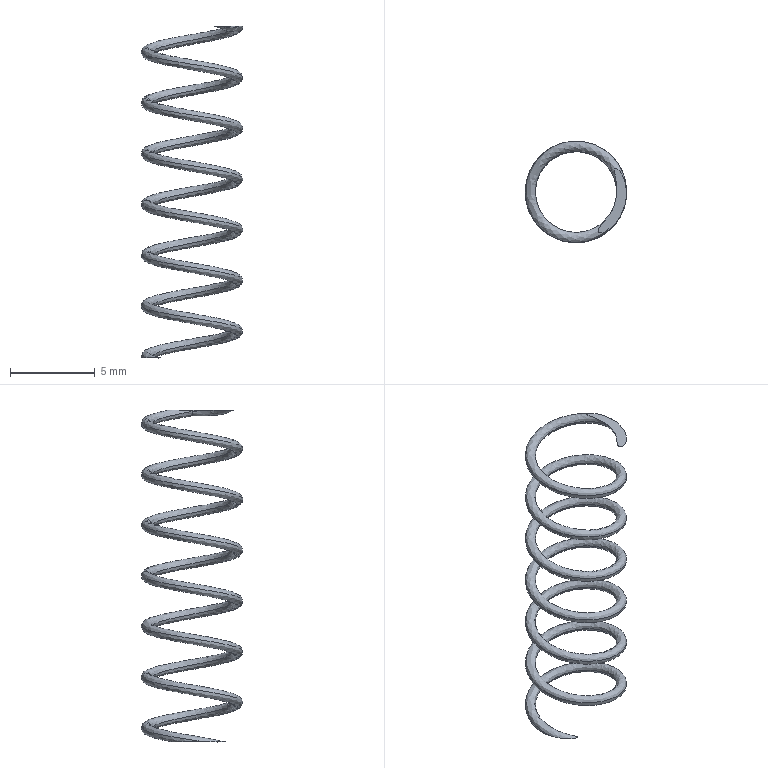Part | SolidWorks | features BaseBody 1 | 1 solid | 7 faces | volume 32.094 mm3 | spline 5 | plane 2